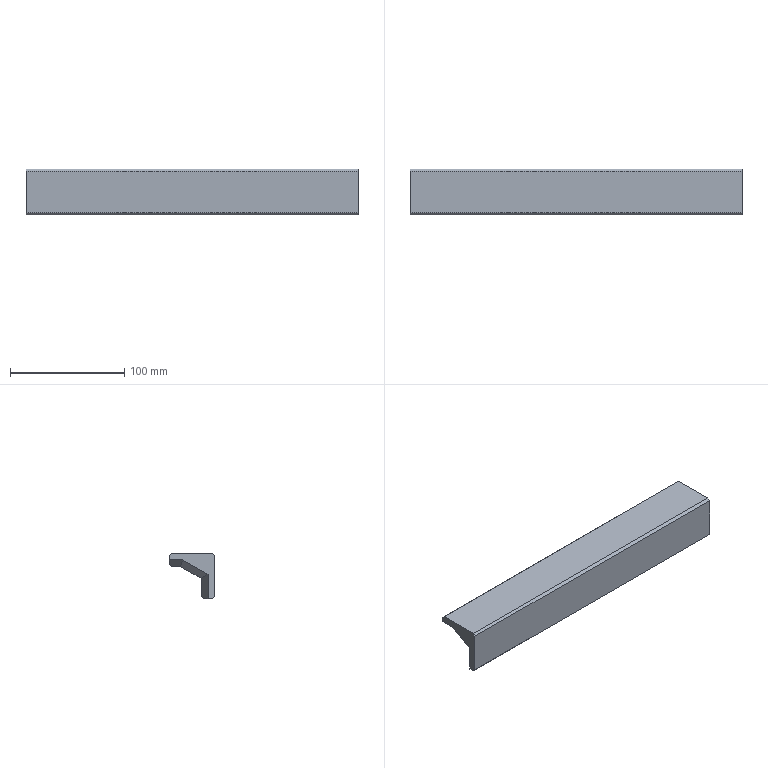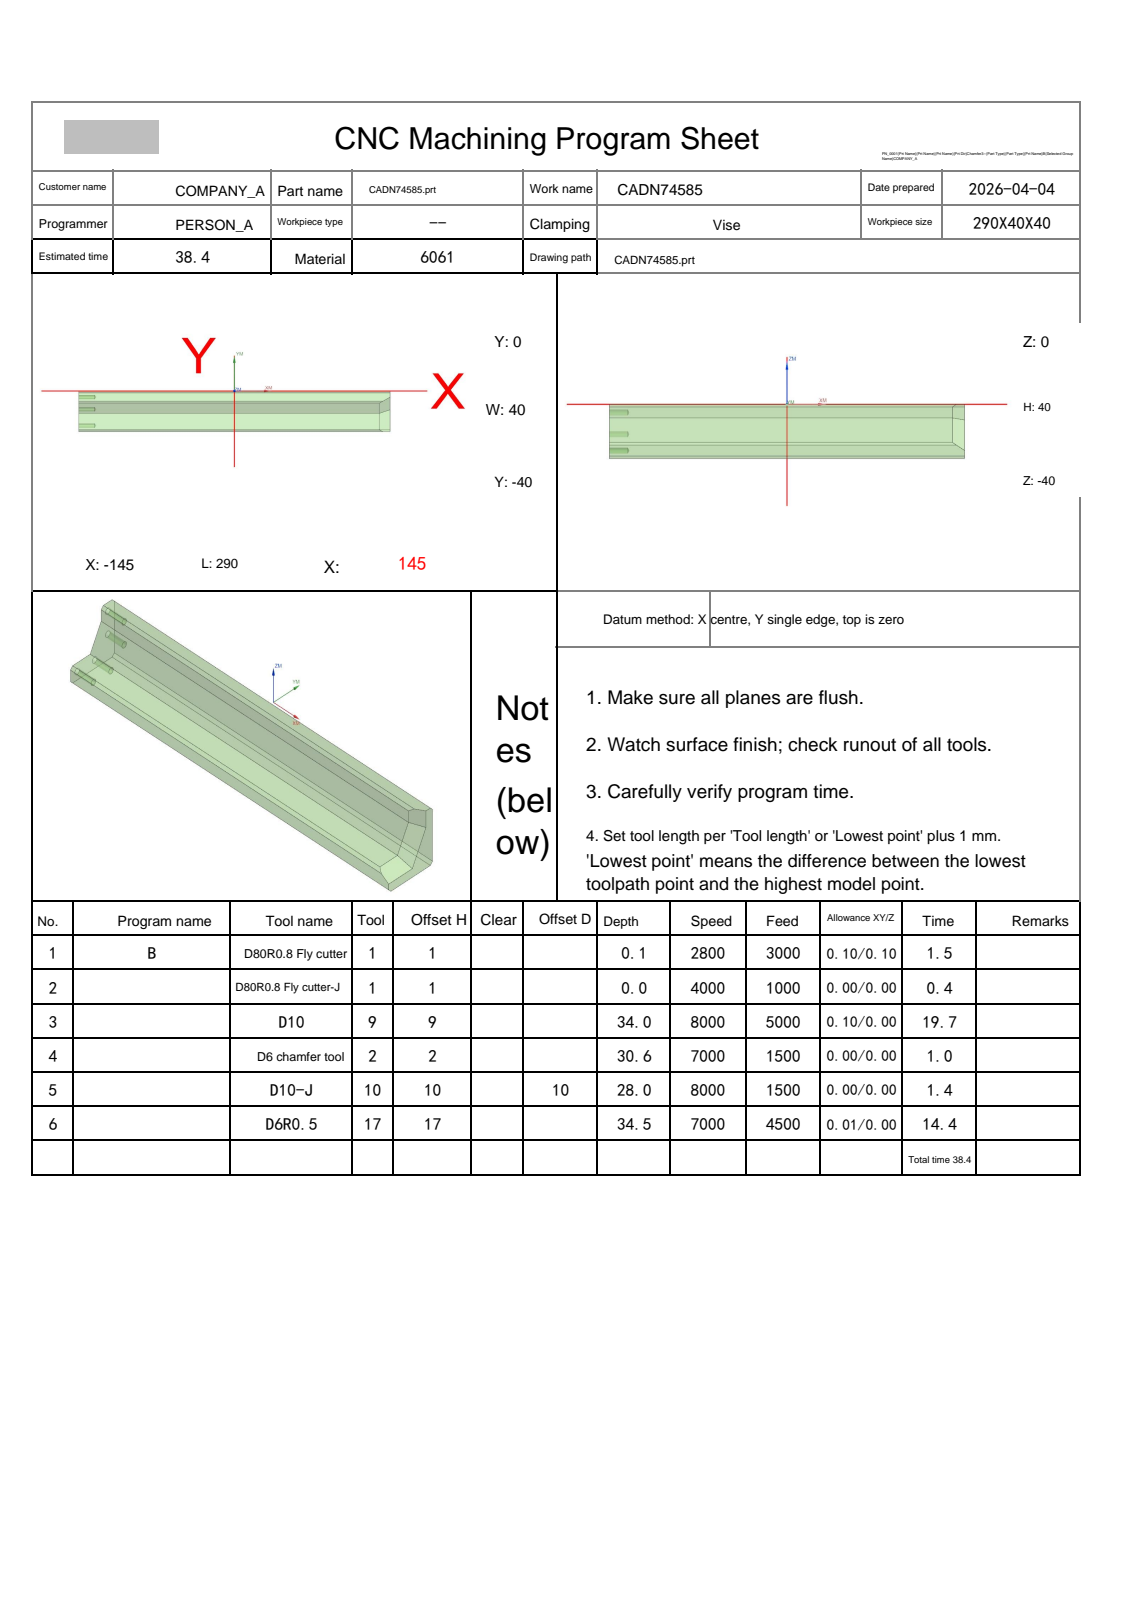NC program | NX | posted by the shop | part box 290 x 40 x 40 mm
Lines 4340 to 6846 of 6846, first 2092 of 2507 lines:
N4 T02 M06
(D6Chamfer D=6. R=0. H=02 ce=0.00 di=0.00)
G00 G90 G54 X-148.9 Y1.516 M03 S6500
G43 H02 Z20.
M08
Z-1.2
G01 Z-2.7 F1000.
G03 X-147.763 Y.7 I1.137 J.384
G01 X147.763
G03 X148.9 Y1.516 I0.0 J1.2
G01 Z-1.2
G00 Z20.
X140.284 Y-13.378
Z-1.2
G01 Z-2.7
G03 X139.204 Y-12.7 I-1.08 J-.522
G01 X-147.763
G03 X-148.9 Y-13.516 I0.0 J-1.2
G01 Z-1.2
G00 Z20.
G00 G90 X142.1 Y-40.6 M03 S7000
Z20.
Z-28.1
G01 Z-30.6 F1000.
X135.
X-145.
X-152.1
Z-28.1
G00 Z20.
G00 G90 X145.99 Y-1.208 M03 S6500
Z20.
Z.13
G01 Z-1.2 F1500.
G03 X145.915 Y-1.548 I1.907 J-.601
G01 X145.905 Y-1.602
X145.928 Y-1.651
X145.966 Y-1.741
X146. Y-2.
Y-6.
X145.967 Y-6.255
X145.87 Y-6.493
X145.716 Y-6.698
X145.514 Y-6.857
X138.848 Y-10.857
X138.6 Y-10.964
X138.534 Y-10.973
X138.51 Y-10.969
X138.495 Y-10.989
X138.435 Y-11.027
X138.393 Y-11.083
Z.314
G00 Z10.
X-145.99 Y-10.792
Z.13
G01 Z-1.2
G03 X-145.915 Y-10.452 I-1.907 J.601
G01 X-145.905 Y-10.398
X-145.928 Y-10.349
X-145.966 Y-10.259
X-146. Y-10.
Y-2.
X-145.966 Y-1.741
X-145.928 Y-1.651
X-145.905 Y-1.602
X-145.915 Y-1.548
G03 X-145.99 Y-1.208 I-1.983 J-.261
G01 Z.13
G00 Z10.
X-145.916 Y-38.379
Z-25.199
G01 Z-29.199
X-145.966 Y-38.259
X-146. Y-38.
Y-24.
X-146.008 Y-23.97
X-146.068 Y-23.884
Z-26.228
G00 Z20.
G91 G28 Z0.0
M05
M09
G91 G28 Z0.0
M01
N5 T10 M06
(D10-J  D=10. R=0. H=10 ce=0.00 di=0.00)
G00 G90 G54 X149.655 Y-10.817 M03 S8000
G43 H10 Z9.5
M08
Z-9.
G01 Z-10. F1000.
G41 D10
X149.533 Y-10.659
G03 X148.344 Y-10.074 I-1.189 J-.915
X147.572 Y-10.287 I0.0 J-1.5
G01 X137.572 Y-16.287
G02 X135. Y-17. I-2.572 J4.287
G01 X-145.
G03 X-146.49 Y-18.327 I0.0 J-1.5
G01 G40 X-146.513 Y-18.526
Z-9.
G00 Z9.5
G00 G90 X142. Y-40.999 M03 S7000
Z14.5
Z-26.5
G01 Z-28. F1500.
G03 X140. Y-39. I-2. J-.001
G01 X-149.1
G02 X-150. Y-38.1 I0.0 J.9
G01 Y-36.133
G02 X-149. Y-35.133 I1. J0.0
G01 X139.1
G03 X140. Y-34.233 I0.0 J.9
G01 Y-32.267
G03 X139. Y-31.267 I-1. J0.0
G01 X-149.1
G02 X-150. Y-30.367 I0.0 J.9
G01 Y-28.4
G02 X-149. Y-27.4 I1. J0.0
G01 X140.
G02 X142. Y-29.399 I0.0 J-2.
G01 Z-26.5
G00 Z14.5
G00 G90 X140.282 Y-27.01 M03 S8000
Z14.5
Z-27.
G01 Z-28. F1000.
G41 D10
X140.083 Y-27.002
X140. Y-27.
X-150.
G03 X-152. Y-28.999 I0.0 J-2.
G01 G40 Y-29.199
Z-27.
G00 Z14.5
G91 G28 Z0.0
M05
M09
G91 G28 Z0.0
M01
N6 T17 M06
(D6R0.5  D=6. R=0.5 H=17 ce=0.01 di=0.00)
G00 G90 G54 X151.954 Y-5.333 M03 S7000
G43 H17 Z14.5
M08
Z-9.6
G01 Z-10.1 F4500.
X147.471 Y-8.027
X146.549 Y-8.581
X136.549 Y-14.581
G02 X135. Y-15.01 I-1.549 J2.581
G01 X-145.
X-146.05
X-146.094 Y-15.008
Z-10.2
X-146.05 Y-15.01
X-145.
X135.
G03 X136.549 Y-14.581 I0.0 J3.01
G01 X146.537 Y-8.588
X146.549 Y-8.582
X147.437 Y-8.05
X147.472 Y-8.027
X147.473 Y-8.028 Z-10.3
X147.437 Y-8.052
X146.538 Y-8.59
X146.482 Y-8.621
X136.549 Y-14.581
G02 X135. Y-15.01 I-1.549 J2.581
G01 X-145.
X-146.05
X-146.095 Y-15.008
Y-15.011 Z-10.348
X-146.096 Y-15.022 Z-10.396
X-146.05 Y-15.024
X135.
G03 X136.553 Y-14.579 I-.028 J3.026
G01 X146.482 Y-8.621
X146.573 Y-8.572
X147.437 Y-8.054
X147.474 Y-8.03
X147.475 Y-8.031 Z-10.484
X146.54 Y-8.592
X146.482 Y-8.621
X137.223 Y-14.176
X136.678 Y-14.551
G02 X135. Y-15.073 I-1.68 J2.443
G01 X-146.05
X-146.098 Y-15.071
X-146.099 Y-15.097 Z-10.527
X-146.1 Y-15.119 Z-10.571
X-146.05 Y-15.121
X135.
G03 X136.678 Y-14.599 I-.003 J2.965
G01 X137.786 Y-13.839
X146.537 Y-8.588
X146.574 Y-8.574
X147.476 Y-8.032
X147.478 Y-8.033 Z-10.658
X147.437 Y-8.06
X146.743 Y-8.476
X146.592 Y-8.565
X146.57 Y-8.568
X138.348 Y-13.502
X136.678 Y-14.648
G02 X135. Y-15.17 I-1.68 J2.443
G01 X-146.05
X-146.1 Y-15.168
Y-15.194 Z-10.702
Y-15.216 Z-10.746
X-146.05 Y-15.219
X135.
G03 X136.678 Y-14.696 I-.003 J2.965
G01 X138.91 Y-13.164
X146.57 Y-8.568
X146.592 Y-8.566
X146.743 Y-8.478
X147.437 Y-8.062
X147.479 Y-8.034
X147.48 Y-8.036 Z-10.833
X147.437 Y-8.064
X146.623 Y-8.55
X146.592 Y-8.566
X146.57 Y-8.568
X139.472 Y-12.827
X136.678 Y-14.745
G02 X135. Y-15.267 I-1.68 J2.443
G01 X-146.05
X-146.1 Y-15.265
Y-15.291 Z-10.877
Y-15.314 Z-10.921
X-146.05 Y-15.316
X135.
G03 X136.678 Y-14.794 I-.003 J2.965
G01 X140.035 Y-12.489
X146.57 Y-8.568
X146.592 Y-8.566
X146.743 Y-8.482
X147.481 Y-8.037
X147.482 Y-8.038 Z-11.008
X147.437 Y-8.067
X146.743 Y-8.484
X146.61 Y-8.558
X146.57 Y-8.568
X140.597 Y-12.152
X136.678 Y-14.842
G02 X135. Y-15.364 I-1.68 J2.443
G01 X-146.05
X-146.1 Y-15.362
Y-15.389 Z-11.052
Y-15.411 Z-11.095
X-146.05 Y-15.413
X135.
G03 X136.678 Y-14.891 I-.003 J2.965
G01 X141.159 Y-11.815
X146.549 Y-8.581
X146.587 Y-8.558
X146.61
X146.743 Y-8.486
X147.437 Y-8.069
X147.483 Y-8.039
X147.484 Y-8.04 Z-11.183
X147.437 Y-8.071
X146.743 Y-8.487
X146.61 Y-8.558
X146.587
X146.549 Y-8.581
X141.721 Y-11.477
X136.678 Y-14.939
G02 X135. Y-15.461 I-1.68 J2.443
G01 X-146.05
X-146.1 Y-15.459
Y-15.486 Z-11.227
Y-15.508 Z-11.27
X-146.05 Y-15.51
X135.
G03 X136.678 Y-14.988 I-.003 J2.965
G01 X142.284 Y-11.14
X146.549 Y-8.581
X146.587 Y-8.558
X146.61
X146.743 Y-8.488
X147.437 Y-8.073
X147.485 Y-8.041
X147.486 Y-8.043 Z-11.358
X147.437 Y-8.075
X146.743 Y-8.489
X146.61 Y-8.558
X146.587
X146.549 Y-8.581
X142.846 Y-10.803
X136.678 Y-15.036
G02 X135. Y-15.558 I-1.68 J2.443
G01 X-146.05
X-146.1 Y-15.556
Y-15.583 Z-11.401
Y-15.605 Z-11.445
X-146.05 Y-15.607
X135.
G03 X136.678 Y-15.085 I-.003 J2.965
G01 X143.408 Y-10.465
X146.549 Y-8.581
X146.587 Y-8.558
X146.61
X146.743 Y-8.49
X147.437 Y-8.077
X147.488 Y-8.044
X147.489 Y-8.045 Z-11.533
X146.743 Y-8.49
X146.624 Y-8.551
X146.603 Y-8.547
X146.549 Y-8.581
X143.97 Y-10.128
X136.678 Y-15.134
G02 X135. Y-15.656 I-1.68 J2.443
G01 X-146.05
X-146.1 Y-15.653
Y-15.68 Z-11.576
Y-15.702 Z-11.62
X-146.05 Y-15.704
X135.
G03 X136.678 Y-15.182 I-.003 J2.965
G01 X144.533 Y-9.791
X146.549 Y-8.581
X146.603 Y-8.547
X146.624 Y-8.551
X146.743 Y-8.49
X147.437 Y-8.081
X147.49 Y-8.046
X147.491 Y-8.047 Z-11.707
X147.437 Y-8.083
X146.743 Y-8.491
X146.624 Y-8.551
X146.603 Y-8.547
X146.549 Y-8.581
X145.095 Y-9.453
X136.678 Y-15.231
G02 X135. Y-15.753 I-1.68 J2.443
G01 X-146.05
X-146.1 Y-15.751
Y-15.777 Z-11.751
Y-15.799 Z-11.795
X-146.05 Y-15.801
X135.
G03 X136.678 Y-15.279 I-.003 J2.965
G01 X145.657 Y-9.116
X146.549 Y-8.581
X146.603 Y-8.547
X146.624 Y-8.551
G03 X147.492 Y-8.048 I-3.924 J7.775
G01 X147.493 Y-8.05 Z-11.882
G02 X146.624 Y-8.551 I-4.828 J7.36
G01 X146.603 Y-8.547
X146.549 Y-8.581
X146.219 Y-8.779
X136.678 Y-15.328
G02 X135. Y-15.85 I-1.68 J2.443
G01 X-146.05
X-146.1 Y-15.848
Y-15.874 Z-11.926
Y-15.896 Z-11.97
X-146.05 Y-15.898
X135.
G03 X136.678 Y-15.376 I-.003 J2.965
G01 X146.602 Y-8.564
G03 X147.495 Y-8.051 I-4.612 J9.049
G01 X147.496 Y-8.052 Z-12.057
G02 X146.633 Y-8.592 I-5.008 J7.049
G01 X136.678 Y-15.425
G02 X135. Y-15.947 I-1.68 J2.443
G01 X-146.05
X-146.1 Y-15.945
Y-15.971 Z-12.101
Y-15.993 Z-12.144
X-146.05 Y-15.996
X135.
G03 X136.678 Y-15.474 I-.003 J2.965
G01 X146.655 Y-8.625
G03 X147.512 Y-8.083 I-3.927 J7.161
G01 X147.524 Y-8.1 Z-12.188
X147.534 Y-8.114 Z-12.232
G02 X146.678 Y-8.658 I-4.667 J6.402
G01 X136.678 Y-15.522
G02 X135. Y-16.044 I-1.68 J2.443
G01 X-146.05
X-146.1 Y-16.042
Y-16.068 Z-12.276
Y-16.091 Z-12.319
X-146.05 Y-16.093
X135.
G03 X136.678 Y-15.571 I-.003 J2.965
G01 X146.636 Y-8.735
G03 X147.556 Y-8.146 I-6.747 J11.544
G01 X147.568 Y-8.162 Z-12.363
X147.579 Y-8.178 Z-12.407
X147.549 Y-8.199
X147.09 Y-8.509
X147.032 Y-8.544
X146.707 Y-8.736
X146.646 Y-8.777
X136.678 Y-15.619
G02 X135. Y-16.141 I-1.68 J2.443
G01 X-146.05
X-146.1 Y-16.139
Y-16.166 Z-12.45
Y-16.188 Z-12.494
X-146.05 Y-16.19
X135.
G03 X136.678 Y-15.668 I-.003 J2.965
G01 X146.655 Y-8.819
X146.729 Y-8.769
X147.09 Y-8.555
X147.595 Y-8.213
X147.596 Y-8.257 Z-12.582
X147.09 Y-8.601
G03 X146.65 Y-8.871 I1.947 J-3.669
G01 X136.678 Y-15.716
G02 X135. Y-16.238 I-1.68 J2.443
G01 X-146.05
X-146.1 Y-16.236
Y-16.263 Z-12.625
Y-16.285 Z-12.669
X-146.05 Y-16.287
X135.
G03 X136.678 Y-15.765 I-.003 J2.965
G01 X146.7 Y-8.886
G02 X147.09 Y-8.648 I2.403 J-3.501
G01 X147.598 Y-8.302
X147.599 Y-8.347 Z-12.756
X147.09 Y-8.694
G03 X146.679 Y-8.949 I2.522 J-4.53
G01 X136.678 Y-15.813
G02 X135. Y-16.336 I-1.68 J2.443
G01 X-146.05
X-146.1 Y-16.333
Y-16.36 Z-12.8
Y-16.382 Z-12.844
X-146.05 Y-16.384
X135.
G03 X136.678 Y-15.862 I-.003 J2.965
G01 X146.652 Y-9.016
G02 X147.09 Y-8.74 I3.675 J-5.354
G01 X147.601 Y-8.392
X147.603 Y-8.437 Z-12.931
X147.09 Y-8.786
G03 X146.656 Y-9.062 I3.569 J-6.109
G01 X136.678 Y-15.911
G02 X135. Y-16.433 I-1.68 J2.443
G01 X-146.05
X-146.1 Y-16.43
Y-16.457 Z-12.975
Y-16.48 Z-13.019
X-146.05 Y-16.481
X135.
G03 X136.678 Y-15.959 I-.003 J2.965
G01 X146.664 Y-9.105
G02 X147.09 Y-8.832 I4.332 J-6.312
G01 X147.519 Y-8.544
X147.605 Y-8.483
X147.608 Y-8.529 Z-13.106
X147.437 Y-8.646
X146.546 Y-9.234
X136.678 Y-16.008
G02 X135. Y-16.53 I-1.68 J2.443
G01 X-146.05
X-146.1 Y-16.528
Y-16.554 Z-13.15
Y-16.576 Z-13.193
X-146.05 Y-16.578
X135.
G03 X136.678 Y-16.056 I-.003 J2.965
G01 X146.667 Y-9.2
X147.437 Y-8.692
X147.609 Y-8.574
X147.61 Y-8.618 Z-13.281
X147.437 Y-8.739
X146.669 Y-9.247
X136.678 Y-16.105
G02 X135. Y-16.627 I-1.68 J2.443
G01 X-146.05
X-146.1 Y-16.625
Y-16.651 Z-13.325
Y-16.673 Z-13.368
X-146.05 Y-16.675
X135.
G03 X136.678 Y-16.153 I-.003 J2.965
G01 X146.678 Y-9.29
X147.437 Y-8.785
X147.611 Y-8.663
X147.613 Y-8.708 Z-13.456
X146.678 Y-9.338
X136.678 Y-16.202
G02 X135. Y-16.724 I-1.68 J2.443
G01 X-146.05
X-146.1 Y-16.722
Y-16.748 Z-13.499
Y-16.77 Z-13.543
X-146.05 Y-16.773
X135.
G03 X136.678 Y-16.251 I-.003 J2.965
G01 X146.678 Y-9.387
X147.437 Y-8.877
X147.615 Y-8.753
X147.617 Y-8.799 Z-13.631
X147.488 Y-8.889
X146.678 Y-9.435
X136.678 Y-16.299
G02 X135. Y-16.821 I-1.68 J2.443
G01 X-146.05
X-146.1 Y-16.819
Y-16.845 Z-13.674
Y-16.868 Z-13.718
X-146.05 Y-16.87
X135.
G03 X136.678 Y-16.348 I-.003 J2.965
G01 X146.678 Y-9.484
X147.557 Y-8.889
X147.62 Y-8.845
X147.622 Y-8.892 Z-13.805
X146.678 Y-9.532
X136.678 Y-16.396
G02 X135. Y-16.918 I-1.68 J2.443
G01 X-146.05
X-146.1 Y-16.916
Y-16.943 Z-13.849
Y-16.965 Z-13.893
X-146.05 Y-16.967
X135.
G03 X136.678 Y-16.445 I-.003 J2.965
G01 X146.678 Y-9.581
X147.437 Y-9.067
X147.621 Y-8.938
X147.62 Y-8.985 Z-13.98
X147.437 Y-9.115
X146.678 Y-9.63
X136.678 Y-16.493
G02 X135. Y-17.015 I-1.68 J2.443
G01 X-146.05
X-146.1 Y-17.013
Y-17.04 Z-14.024
Y-17.062 Z-14.068
X-146.05 Y-17.064
X135.
G03 X136.678 Y-16.542 I-.003 J2.965
G01 X146.678 Y-9.678
X147.437 Y-9.162
X147.62 Y-9.033
Y-9.08 Z-14.155
X147.437 Y-9.209
X146.678 Y-9.727
X136.678 Y-16.59
G02 X135. Y-17.113 I-1.68 J2.443
G01 X-146.05
X-146.1 Y-17.11
Y-17.137 Z-14.199
Y-17.159 Z-14.242
X-146.05 Y-17.161
X135.
G03 X136.678 Y-16.639 I-.003 J2.965
G01 X146.678 Y-9.775
X147.471 Y-9.234
X147.62 Y-9.129
X147.621 Y-9.178 Z-14.33
X147.543 Y-9.234
X146.678 Y-9.824
X136.678 Y-16.688
G02 X135. Y-17.21 I-1.68 J2.443
G01 X-146.05
X-146.1 Y-17.208
Y-17.234 Z-14.374
Y-17.256 Z-14.417
X-146.05 Y-17.258
X135.
G03 X136.678 Y-16.736 I-.003 J2.965
G01 X146.678 Y-9.872
X147.622 Y-9.228
X147.621 Y-9.275 Z-14.505
X147.437 Y-9.402
X146.678 Y-9.921
X136.678 Y-16.785
G02 X135. Y-17.307 I-1.68 J2.443
G01 X-146.05
X-146.1 Y-17.305
Y-17.331 Z-14.548
Y-17.353 Z-14.592
X-146.05 Y-17.355
X135.
G03 X136.678 Y-16.833 I-.003 J2.965
G01 X146.678 Y-9.97
X147.437 Y-9.45
X147.62 Y-9.322
Y-9.37 Z-14.68
X147.437 Y-9.499
X146.678 Y-10.018
X136.678 Y-16.882
G02 X135. Y-17.404 I-1.68 J2.443
G01 X-146.05
X-146.1 Y-17.402
Y-17.428 Z-14.723
Y-17.45 Z-14.767
X-146.05 Y-17.453
X135.
G03 X136.678 Y-16.93 I-.003 J2.965
G01 X146.678 Y-10.067
X147.437 Y-9.547
X147.62 Y-9.418
Y-9.467 Z-14.854
X147.461 Y-9.579
X146.678 Y-10.115
X136.678 Y-16.979
G02 X135. Y-17.501 I-1.68 J2.443
G01 X-146.05
X-146.1 Y-17.499
Y-17.525 Z-14.898
Y-17.547 Z-14.942
X-146.05 Y-17.55
X135.
G03 X136.678 Y-17.028 I-.003 J2.965
G01 X146.678 Y-10.164
X147.532 Y-9.579
X147.62 Y-9.516
X147.621 Y-9.566 Z-15.029
X146.678 Y-10.212
X136.678 Y-17.076
G02 X135. Y-17.598 I-1.68 J2.443
G01 X-146.05
X-146.1 Y-17.596
Y-17.622 Z-15.073
Y-17.645 Z-15.117
X-146.05 Y-17.647
X135.
G03 X136.678 Y-17.125 I-.003 J2.965
G01 X146.678 Y-10.261
X147.437 Y-9.74
X147.62 Y-9.614
Y-9.661 Z-15.204
X147.437 Y-9.789
X146.678 Y-10.309
X136.678 Y-17.173
G02 X135. Y-17.695 I-1.68 J2.443
G01 X-146.05
X-146.1 Y-17.693
Y-17.72 Z-15.248
Y-17.742 Z-15.291
X-146.05 Y-17.744
X135.
G03 X136.678 Y-17.222 I-.003 J2.965
G01 X146.678 Y-10.358
X147.437 Y-9.837
X147.619 Y-9.709
Y-9.757 Z-15.379
X147.437 Y-9.886
X146.678 Y-10.407
X136.678 Y-17.27
G02 X135. Y-17.792 I-1.68 J2.443
G01 X-146.05
X-146.1 Y-17.79
Y-17.817 Z-15.423
Y-17.839 Z-15.466
X-146.05 Y-17.841
X135.
G03 X136.678 Y-17.319 I-.003 J2.965
G01 X146.678 Y-10.455
X147.452 Y-9.924
X147.619 Y-9.806
Y-9.855 Z-15.554
X147.522 Y-9.924
X146.678 Y-10.504
X136.678 Y-17.368
G02 X135. Y-17.89 I-1.68 J2.443
G01 X-146.05
X-146.1 Y-17.887
Y-17.914 Z-15.597
Y-17.936 Z-15.641
X-146.05 Y-17.938
X135.
G03 X136.678 Y-17.416 I-.003 J2.965
G01 X146.678 Y-10.552
X147.593 Y-9.924
X147.62 Y-9.904
Y-9.953 Z-15.729
X147.437 Y-10.08
X146.678 Y-10.601
X136.678 Y-17.465
G02 X135. Y-17.987 I-1.68 J2.443
G01 X-146.05
X-146.1 Y-17.985
Y-18.011 Z-15.772
Y-18.033 Z-15.816
X-146.05 Y-18.035
X135.
G03 X136.678 Y-17.513 I-.003 J2.965
G01 X146.678 Y-10.649
X147.437 Y-10.128
X147.619 Y-10.
Y-10.048 Z-15.903
X147.437 Y-10.177
X146.678 Y-10.698
X136.678 Y-17.562
G02 X135. Y-18.084 I-1.68 J2.443
G01 X-146.05
X-146.1 Y-18.082
Y-18.108 Z-15.947
Y-18.13 Z-15.991
X-146.05 Y-18.132
X135.
G03 X136.678 Y-17.61 I-.003 J2.965
G01 X146.678 Y-10.747
X147.437 Y-10.225
X147.619 Y-10.097
Y-10.145 Z-16.078
X147.444 Y-10.269
X146.678 Y-10.795
X136.678 Y-17.659
G02 X135. Y-18.181 I-1.68 J2.443
G01 X-146.05
X-146.1 Y-18.179
Y-18.205 Z-16.122
Y-18.227 Z-16.166
X-146.05 Y-18.23
X135.
G03 X136.678 Y-17.707 I-.003 J2.965
G01 X146.678 Y-10.844
X147.515 Y-10.269
X147.619 Y-10.194
X147.62 Y-10.244 Z-16.253
X147.586 Y-10.269
X146.678 Y-10.892
X136.678 Y-17.756
G02 X135. Y-18.278 I-1.68 J2.443
G01 X-146.05
X-146.1 Y-18.276
Y-18.302 Z-16.297
Y-18.325 Z-16.34
X-146.05 Y-18.327
X135.
G03 X136.678 Y-17.805 I-.003 J2.965
G01 X146.678 Y-10.941
X147.437 Y-10.42
X147.62 Y-10.293
X147.619 Y-10.34 Z-16.428
X147.437 Y-10.468
X146.678 Y-10.989
X136.678 Y-17.853
G02 X135. Y-18.375 I-1.68 J2.443
G01 X-146.05
X-146.1 Y-18.373
Y-18.4 Z-16.472
Y-18.422 Z-16.515
X-146.05 Y-18.424
X135.
G03 X136.678 Y-17.902 I-.003 J2.965
G01 X146.678 Y-11.038
X147.437 Y-10.517
X147.619 Y-10.388
Y-10.436 Z-16.603
X147.437 Y-10.565
X146.678 Y-11.087
X136.678 Y-17.95
G02 X135. Y-18.472 I-1.68 J2.443
G01 X-146.05
X-146.1 Y-18.47
Y-18.497 Z-16.646
Y-18.519 Z-16.69
X-146.05 Y-18.521
X135.
G03 X136.678 Y-17.999 I-.003 J2.965
G01 X146.678 Y-11.135
X147.437 Y-10.614
X147.619 Y-10.485
Y-10.534 Z-16.778
X147.507 Y-10.614
X146.678 Y-11.184
X136.678 Y-18.047
G02 X135. Y-18.569 I-1.68 J2.443
G01 X-146.05
X-146.1 Y-18.567
Y-18.594 Z-16.821
Y-18.616 Z-16.865
X-146.05 Y-18.618
X135.
G03 X136.678 Y-18.096 I-.003 J2.965
G01 X146.678 Y-11.232
X147.578 Y-10.614
X147.62 Y-10.584
Y-10.633 Z-16.952
X147.437 Y-10.76
X146.678 Y-11.281
X136.678 Y-18.145
G02 X135. Y-18.667 I-1.68 J2.443
G01 X-146.05
X-146.1 Y-18.664
Y-18.691 Z-16.996
Y-18.713 Z-17.04
X-146.05 Y-18.715
X135.
G03 X136.678 Y-18.193 I-.003 J2.965
G01 X146.678 Y-11.329
X147.437 Y-10.808
X147.619 Y-10.68
Y-10.728 Z-17.127
X147.437 Y-10.857
X146.678 Y-11.378
X136.678 Y-18.242
G02 X135. Y-18.764 I-1.68 J2.443
G01 X-146.05
X-146.1 Y-18.762
Y-18.788 Z-17.171
Y-18.81 Z-17.215
X-146.05 Y-18.812
X135.
G03 X136.678 Y-18.29 I-.003 J2.965
G01 X146.678 Y-11.426
X147.437 Y-10.905
X147.619 Y-10.776
Y-10.825 Z-17.302
X147.437 Y-10.954
X146.678 Y-11.475
X136.678 Y-18.339
G02 X135. Y-18.861 I-1.68 J2.443
G01 X-146.05
X-146.1 Y-18.859
Y-18.885 Z-17.346
Y-18.907 Z-17.389
X-146.05 Y-18.909
X135.
G03 X136.678 Y-18.387 I-.003 J2.965
G01 X146.678 Y-11.524
X147.5 Y-10.959
X147.619 Y-10.874
X147.62 Y-10.924 Z-17.477
X147.571 Y-10.959
X146.678 Y-11.572
X136.678 Y-18.436
G02 X135. Y-18.958 I-1.68 J2.443
G01 X-146.05
X-146.1 Y-18.956
Y-18.982 Z-17.521
Y-19.004 Z-17.564
X-146.05 Y-19.007
X135.
G03 X136.678 Y-18.484 I-.003 J2.965
G01 X146.678 Y-11.621
X147.62 Y-10.973
X147.619 Y-11.02 Z-17.652
X147.437 Y-11.148
X146.678 Y-11.669
X136.678 Y-18.533
G02 X135. Y-19.055 I-1.68 J2.443
G01 X-146.05
X-146.1 Y-19.053
Y-19.079 Z-17.695
Y-19.102 Z-17.739
X-146.05 Y-19.104
X135.
G03 X136.678 Y-18.582 I-.003 J2.965
G01 X146.678 Y-11.718
X147.437 Y-11.197
X147.619 Y-11.068
Y-11.116 Z-17.826
X147.437 Y-11.245
X146.678 Y-11.766
X136.678 Y-18.63
G02 X135. Y-19.152 I-1.68 J2.443
G01 X-146.05
X-146.1 Y-19.15
Y-19.177 Z-17.87
Y-19.199 Z-17.914
X-146.05 Y-19.201
X135.
G03 X136.678 Y-18.679 I-.003 J2.965
G01 X146.678 Y-11.815
X147.437 Y-11.294
X147.619 Y-11.165
Y-11.214 Z-18.001
X147.493 Y-11.304
X146.678 Y-11.864
X136.678 Y-18.727
G02 X135. Y-19.249 I-1.68 J2.443
G01 X-146.05
X-146.1 Y-19.247
Y-19.274 Z-18.045
Y-19.296 Z-18.089
X-146.05 Y-19.298
X135.
G03 X136.678 Y-18.776 I-.003 J2.965
G01 X146.678 Y-11.912
X147.563 Y-11.304
X147.62 Y-11.263
X147.621 Y-11.313 Z-18.176
X146.678 Y-11.961
X136.678 Y-18.824
G02 X135. Y-19.347 I-1.68 J2.443
G01 X-146.05
X-146.1 Y-19.344
Y-19.371 Z-18.22
Y-19.393 Z-18.264
X-146.05 Y-19.395
X135.
G03 X136.678 Y-18.873 I-.003 J2.965
G01 X146.678 Y-12.009
X147.437 Y-11.488
X147.62 Y-11.36
X147.619 Y-11.408 Z-18.351
X147.437 Y-11.537
X146.678 Y-12.058
X136.678 Y-18.922
G02 X135. Y-19.444 I-1.68 J2.443
G01 X-146.05
X-146.1 Y-19.441
Y-19.468 Z-18.395
Y-19.49 Z-18.438
X-146.05 Y-19.492
X135.
G03 X136.678 Y-18.97 I-.003 J2.965
G01 X146.678 Y-12.106
X147.437 Y-11.585
X147.619 Y-11.456
Y-11.505 Z-18.526
X147.437 Y-11.634
X146.678 Y-12.155
X136.678 Y-19.019
G02 X135. Y-19.541 I-1.68 J2.443
G01 X-146.05
X-146.1 Y-19.539
Y-19.565 Z-18.57
Y-19.588 Z-18.613
X-146.05 Y-19.589
X135.
G03 X136.678 Y-19.067 I-.003 J2.965
G01 X146.678 Y-12.203
X147.485 Y-11.649
X147.619 Y-11.554
X147.62 Y-11.603 Z-18.701
X147.556 Y-11.649
X146.678 Y-12.252
X136.678 Y-19.116
G02 X135. Y-19.638 I-1.68 J2.443
G01 X-146.05
X-146.1 Y-19.636
Y-19.662 Z-18.744
Y-19.684 Z-18.788
X-146.05 Y-19.686
X135.
G03 X136.678 Y-19.164 I-.003 J2.965
G01 X146.678 Y-12.301
X147.621 Y-11.653
X147.62 Y-11.7 Z-18.875
X147.437 Y-11.828
X146.678 Y-12.349
X136.678 Y-19.213
G02 X135. Y-19.735 I-1.68 J2.443
G01 X-146.05
X-146.1 Y-19.733
Y-19.759 Z-18.919
Y-19.781 Z-18.963
X-146.05 Y-19.784
X135.
G03 X136.678 Y-19.262 I-.003 J2.965
G01 X146.678 Y-12.398
X147.437 Y-11.877
X147.619 Y-11.748
Y-11.796 Z-19.05
X147.437 Y-11.925
X146.678 Y-12.446
X136.678 Y-19.31
G02 X135. Y-19.832 I-1.68 J2.443
G01 X-146.05
X-146.1 Y-19.83
Y-19.856 Z-19.094
Y-19.879 Z-19.138
X-146.05 Y-19.881
X135.
G03 X136.678 Y-19.359 I-.003 J2.965
G01 X146.678 Y-12.495
X147.437 Y-11.974
X147.619 Y-11.845
Y-11.894 Z-19.225
X147.478 Y-11.994
X146.678 Y-12.543
X136.678 Y-19.407
G02 X135. Y-19.929 I-1.68 J2.443
G01 X-146.05
X-146.1 Y-19.927
Y-19.954 Z-19.269
Y-19.976 Z-19.313
X-146.05 Y-19.978
X135.
G03 X136.678 Y-19.456 I-.003 J2.965
G01 X146.678 Y-12.592
X147.549 Y-11.994
X147.62 Y-11.943
X147.621 Y-11.993 Z-19.4
X146.678 Y-12.641
X136.678 Y-19.504
G02 X135. Y-20.026 I-1.68 J2.443
G01 X-146.05
X-146.1 Y-20.024
Y-20.051 Z-19.444
Y-20.073 Z-19.487
X-146.05 Y-20.075
X135.
G03 X136.678 Y-19.553 I-.003 J2.965
G01 X146.678 Y-12.689
X147.437 Y-12.168
X147.62 Y-12.04
X147.619 Y-12.088 Z-19.575
X147.437 Y-12.216
X146.678 Y-12.738
X136.678 Y-19.601
G02 X135. Y-20.124 I-1.68 J2.443
G01 X-146.05
X-146.1 Y-20.121
Y-20.148 Z-19.619
Y-20.17 Z-19.662
X-146.05 Y-20.172
X135.
G03 X136.678 Y-19.65 I-.003 J2.965
G01 X146.678 Y-12.786
X147.437 Y-12.265
X147.619 Y-12.136
Y-12.185 Z-19.75
X147.437 Y-12.314
X146.678 Y-12.835
X136.678 Y-19.699
G02 X135. Y-20.221 I-1.68 J2.443
G01 X-146.05
X-146.1 Y-20.219
Y-20.245 Z-19.793
Y-20.267 Z-19.837
X-146.05 Y-20.269
X135.
G03 X136.678 Y-19.747 I-.003 J2.965
G01 X146.678 Y-12.883
X147.47 Y-12.339
X147.619 Y-12.233
X147.62 Y-12.283 Z-19.924
X147.541 Y-12.339
X146.678 Y-12.932
X136.678 Y-19.796
G02 X135. Y-20.318 I-1.68 J2.443
G01 X-146.05
X-146.1 Y-20.316
Y-20.342 Z-19.968
Y-20.364 Z-20.012
X-146.05 Y-20.366
X135.
G03 X136.678 Y-19.844 I-.003 J2.965
G01 X146.678 Y-12.981
X147.621 Y-12.333
X147.62 Y-12.38 Z-20.099
X147.437 Y-12.508
X146.397 Y-13.222
X136.678 Y-19.893
G02 X135. Y-20.415 I-1.68 J2.443
G01 X-146.05
X-146.1 Y-20.413
Y-20.439 Z-20.143
Y-20.461 Z-20.187
X-146.05 Y-20.463
X135.
G03 X136.678 Y-19.941 I-.003 J2.965
G01 X146.678 Y-13.078
X147.437 Y-12.556
X147.619 Y-12.428
Y-12.476 Z-20.274
X147.437 Y-12.605
X146.678 Y-13.126
X136.678 Y-19.99
G02 X135. Y-20.512 I-1.68 J2.443
G01 X-146.05
X-146.1 Y-20.51
Y-20.536 Z-20.318
Y-20.558 Z-20.362
X-146.05 Y-20.561
X135.
G03 X136.678 Y-20.039 I-.003 J2.965
G01 X146.678 Y-13.175
X147.437 Y-12.654
X147.619 Y-12.525
Y-12.573 Z-20.449
X147.463 Y-12.684
X146.678 Y-13.223
X136.678 Y-20.087
G02 X135. Y-20.609 I-1.68 J2.443
G01 X-146.05
X-146.1 Y-20.607
Y-20.633 Z-20.493
Y-20.656 Z-20.536
X-146.05 Y-20.658
X135.
G03 X136.678 Y-20.136 I-.003 J2.965
G01 X146.678 Y-13.272
X147.534 Y-12.684
X147.62 Y-12.623
X147.621 Y-12.673 Z-20.624
X146.678 Y-13.32
X136.678 Y-20.184
G02 X135. Y-20.706 I-1.68 J2.443
G01 X-146.05
X-146.1 Y-20.704
Y-20.731 Z-20.668
Y-20.753 Z-20.711
X-146.05 Y-20.755
X135.
G03 X136.678 Y-20.233 I-.003 J2.965
G01 X146.678 Y-13.369
X147.437 Y-12.848
X147.62 Y-12.72
X147.619 Y-12.768 Z-20.799
X147.437 Y-12.896
X146.678 Y-13.418
X136.678 Y-20.281
G02 X135. Y-20.803 I-1.68 J2.443
G01 X-146.05
X-146.1 Y-20.801
Y-20.828 Z-20.842
Y-20.85 Z-20.886
X-146.05 Y-20.852
X135.
G03 X136.678 Y-20.33 I-.003 J2.965
G01 X146.678 Y-13.466
X147.437 Y-12.945
X147.619 Y-12.816
Y-12.865 Z-20.973
X147.437 Y-12.993
X146.678 Y-13.515
X136.678 Y-20.379
G02 X135. Y-20.901 I-1.68 J2.443
G01 X-146.05
X-146.1 Y-20.898
Y-20.925 Z-21.017
Y-20.947 Z-21.061
X-146.05 Y-20.949
X135.
G03 X136.678 Y-20.427 I-.003 J2.965
G01 X146.678 Y-13.563
X147.456 Y-13.029
X147.619 Y-12.913
Y-12.963 Z-21.148
X147.526 Y-13.029
X146.678 Y-13.612
X136.678 Y-20.476
G02 X135. Y-20.998 I-1.68 J2.443
G01 X-146.05
X-146.1 Y-20.996
Y-21.022 Z-21.192
Y-21.044 Z-21.236
X-146.05 Y-21.046
X135.
G03 X136.678 Y-20.524 I-.003 J2.965
G01 X146.678 Y-13.66
X147.62 Y-13.012
Y-13.061 Z-21.323
X147.437 Y-13.188
X146.678 Y-13.709
X136.678 Y-20.573
G02 X135. Y-21.095 I-1.68 J2.443
G01 X-146.05
X-146.1 Y-21.093
Y-21.119 Z-21.367
Y-21.141 Z-21.411
X-146.05 Y-21.143
X135.
G03 X136.678 Y-20.621 I-.003 J2.965
G01 X146.678 Y-13.758
X147.437 Y-13.236
X147.619 Y-13.108
Y-13.156 Z-21.498
X147.437 Y-13.285
X146.678 Y-13.806
X136.678 Y-20.67
G02 X135. Y-21.192 I-1.68 J2.443
G01 X-146.05
X-146.1 Y-21.19
Y-21.216 Z-21.542
Y-21.238 Z-21.585
X-146.05 Y-21.241
X135.
G03 X136.678 Y-20.718 I-.003 J2.965
G01 X146.678 Y-13.855
X147.437 Y-13.333
X147.619 Y-13.205
Y-13.253 Z-21.673
X147.448 Y-13.375
X146.678 Y-13.903
X136.678 Y-20.767
G02 X135. Y-21.289 I-1.68 J2.443
G01 X-146.05
X-146.1 Y-21.287
Y-21.313 Z-21.716
Y-21.335 Z-21.76
X-146.05 Y-21.338
X135.
G03 X136.678 Y-20.816 I-.003 J2.965
G01 X146.678 Y-13.952
X147.519 Y-13.375
X147.619 Y-13.302
X147.62 Y-13.352 Z-21.848
X147.59 Y-13.375
X146.678 Y-14.
X136.678 Y-20.864
G02 X135. Y-21.386 I-1.68 J2.443
G01 X-146.05
X-146.1 Y-21.384
Y-21.41 Z-21.891
Y-21.433 Z-21.935
X-146.05 Y-21.435
X135.
G03 X136.678 Y-20.913 I-.003 J2.965
G01 X146.678 Y-14.049
X147.437 Y-13.528
X147.62 Y-13.401
X147.619 Y-13.448 Z-22.022
X147.437 Y-13.576
X146.678 Y-14.097
X136.678 Y-20.961
G02 X135. Y-21.483 I-1.68 J2.443
G01 X-146.05
X-146.1 Y-21.481
Y-21.508 Z-22.066
Y-21.53 Z-22.11
X-146.05 Y-21.532
X135.
G03 X136.678 Y-21.01 I-.003 J2.965
G01 X146.678 Y-14.146
X147.437 Y-13.625
X147.619 Y-13.496
Y-13.544 Z-22.197
X147.437 Y-13.673
X146.678 Y-14.195
X136.678 Y-21.058
G02 X135. Y-21.58 I-1.68 J2.443
G01 X-146.05
X-146.1 Y-21.578
Y-21.605 Z-22.241
Y-21.627 Z-22.285
X-146.05 Y-21.629
X135.
G03 X136.678 Y-21.107 I-.003 J2.965
G01 X146.678 Y-14.243
X147.441 Y-13.72
X147.619 Y-13.593
Y-13.642 Z-22.372
X147.512 Y-13.72
X146.678 Y-14.292
X136.678 Y-21.156
G02 X135. Y-21.678 I-1.68 J2.443
G01 X-146.05
X-146.1 Y-21.675
Y-21.702 Z-22.416
Y-21.724 Z-22.46
X-146.05 Y-21.726
X135.
G03 X136.678 Y-21.204 I-.003 J2.965
G01 X146.678 Y-14.34
X147.582 Y-13.72
X147.62 Y-13.692
Y-13.741 Z-22.547
X147.437 Y-13.868
X146.678 Y-14.389
X136.678 Y-21.253
G02 X135. Y-21.775 I-1.68 J2.443
G01 X-146.05
X-146.1 Y-21.773
Y-21.799 Z-22.591
Y-21.821 Z-22.634
X-146.05 Y-21.823
X135.
G03 X136.678 Y-21.301 I-.003 J2.965
G01 X146.678 Y-14.437
X147.437 Y-13.916
X147.619 Y-13.788
Y-13.836 Z-22.722
X147.437 Y-13.965
X146.678 Y-14.486
X136.678 Y-21.35
G02 X135. Y-21.872 I-1.68 J2.443
G01 X-146.05
X-146.1 Y-21.87
Y-21.896 Z-22.765
Y-21.918 Z-22.809
X-146.05 Y-21.92
X135.
G03 X136.678 Y-21.398 I-.003 J2.965
G01 X146.678 Y-14.535
X147.437 Y-14.013
X147.619 Y-13.884
Y-13.933 Z-22.897
X147.437 Y-14.062
X146.678 Y-14.583
X136.678 Y-21.447
G02 X135. Y-21.969 I-1.68 J2.443
G01 X-146.05
X-146.1 Y-21.967
Y-21.993 Z-22.94
Y-22.015 Z-22.984
X-146.05 Y-22.018
X135.
G03 X136.678 Y-21.495 I-.003 J2.965
G01 X146.678 Y-14.632
X147.504 Y-14.065
X147.619 Y-13.982
X147.62 Y-14.032 Z-23.071
X147.575 Y-14.065
X146.678 Y-14.68
X136.678 Y-21.544
G02 X135. Y-22.066 I-1.68 J2.443
G01 X-146.05
X-146.1 Y-22.064
Y-22.09 Z-23.115
Y-22.113 Z-23.159
X-146.05 Y-22.115
X135.
G03 X136.678 Y-21.593 I-.003 J2.965
G01 X146.678 Y-14.729
X147.437 Y-14.208
X147.62 Y-14.081
X147.619 Y-14.128 Z-23.246
X147.437 Y-14.256
X146.678 Y-14.777
X136.678 Y-21.641
G02 X135. Y-22.163 I-1.68 J2.443
G01 X-146.05
X-146.1 Y-22.161
Y-22.188 Z-23.29
Y-22.21 Z-23.334
X-146.05 Y-22.212
X135.
G03 X136.678 Y-21.69 I-.003 J2.965
G01 X146.678 Y-14.826
X147.437 Y-14.305
X147.619 Y-14.176
Y-14.224 Z-23.421
X147.437 Y-14.353
X146.678 Y-14.875
X136.678 Y-21.738
G02 X135. Y-22.26 I-1.68 J2.443
G01 X-146.05
X-146.1 Y-22.258
Y-22.285 Z-23.465
Y-22.307 Z-23.509
X-146.05 Y-22.309
X135.
G03 X136.678 Y-21.787 I-.003 J2.965
G01 X146.678 Y-14.923
X147.437 Y-14.402
X147.619 Y-14.273
Y-14.322 Z-23.596
X147.497 Y-14.41
X146.678 Y-14.972
X136.678 Y-21.835
G02 X135. Y-22.357 I-1.68 J2.443
G01 X-146.05
X-146.1 Y-22.355
Y-22.382 Z-23.64
Y-22.404 Z-23.683
X-146.05 Y-22.406
X135.
G03 X136.678 Y-21.884 I-.003 J2.965
G01 X146.678 Y-15.02
X147.568 Y-14.41
X147.62 Y-14.372
X147.621 Y-14.421 Z-23.771
X146.678 Y-15.069
X136.678 Y-21.933
G02 X135. Y-22.455 I-1.68 J2.443
G01 X-146.05
X-146.1 Y-22.452
Y-22.479 Z-23.814
Y-22.501 Z-23.858
X-146.05 Y-22.503
X135.
G03 X136.678 Y-21.981 I-.003 J2.965
G01 X146.678 Y-15.117
X147.437 Y-14.596
X147.62 Y-14.468
X147.619 Y-14.516 Z-23.946
X147.437 Y-14.645
X146.678 Y-15.166
X136.678 Y-22.03
G02 X135. Y-22.552 I-1.68 J2.443
G01 X-146.05
X-146.1 Y-22.55
Y-22.576 Z-23.989
Y-22.598 Z-24.033
X-146.05 Y-22.6
X135.
G03 X136.678 Y-22.078 I-.003 J2.965
G01 X146.678 Y-15.214
X147.437 Y-14.693
X147.619 Y-14.564
Y-14.613 Z-24.12
X147.437 Y-14.742
X146.678 Y-15.263
X136.678 Y-22.127
G02 X135. Y-22.649 I-1.68 J2.443
G01 X-146.05
X-146.1 Y-22.647
Y-22.673 Z-24.164
Y-22.696 Z-24.208
X-146.05 Y-22.697
X135.
G03 X136.678 Y-22.175 I-.003 J2.965
G01 X146.678 Y-15.312
X147.489 Y-14.755
X147.619 Y-14.662
X147.62 Y-14.711 Z-24.295
X147.56 Y-14.755
X146.678 Y-15.36
X136.678 Y-22.224
G02 X135. Y-22.746 I-1.68 J2.443
G01 X-146.05
X-146.1 Y-22.744
Y-22.77 Z-24.339
Y-22.792 Z-24.383
X-146.05 Y-22.795
X135.
G03 X136.678 Y-22.273 I-.003 J2.965
G01 X146.678 Y-15.409
X147.621 Y-14.761
X147.62 Y-14.808 Z-24.47
X147.437 Y-14.936
X146.678 Y-15.457
X136.678 Y-22.321
G02 X135. Y-22.843 I-1.68 J2.443
G01 X-146.05
X-146.1 Y-22.841
Y-22.867 Z-24.514
Y-22.89 Z-24.558
X-146.05 Y-22.892
X135.
G03 X136.678 Y-22.37 I-.003 J2.965
G01 X146.678 Y-15.506
X147.437 Y-14.985
X147.619 Y-14.856
Y-14.904 Z-24.645
X147.437 Y-15.033
X146.678 Y-15.554
X136.678 Y-22.418
G02 X135. Y-22.94 I-1.68 J2.443
G01 X-146.05
X-146.1 Y-22.938
Y-22.965 Z-24.689
Y-22.987 Z-24.732
X-146.05 Y-22.989
X135.
G03 X136.678 Y-22.467 I-.003 J2.965
G01 X146.678 Y-15.603
X147.437 Y-15.082
X147.619 Y-14.953
Y-15.002 Z-24.82
X147.482 Y-15.1
X146.678 Y-15.652
X136.678 Y-22.515
G02 X135. Y-23.037 I-1.68 J2.443
G01 X-146.05
X-146.1 Y-23.036
Y-23.062 Z-24.863
Y-23.084 Z-24.907
X-146.05 Y-23.086
X135.
G03 X136.678 Y-22.564 I-.003 J2.965
G01 X146.678 Y-15.7
X147.553 Y-15.1
X147.62 Y-15.051
X147.621 Y-15.101 Z-24.995
X146.678 Y-15.749
X136.678 Y-22.612
G02 X135. Y-23.135 I-1.68 J2.443
G01 X-146.05
X-146.1 Y-23.132
Y-23.159 Z-25.038
Y-23.181 Z-25.082
X-146.05 Y-23.183
X135.
G03 X136.678 Y-22.661 I-.003 J2.965
G01 X146.678 Y-15.797
X147.437 Y-15.276
X147.62 Y-15.148
X147.619 Y-15.196 Z-25.169
X147.437 Y-15.325
X146.678 Y-15.846
X136.678 Y-22.71
G02 X135. Y-23.232 I-1.68 J2.443
G01 X-146.05
X-146.1 Y-23.229
Y-23.256 Z-25.213
Y-23.278 Z-25.257
X-146.05 Y-23.28
X135.
G03 X136.678 Y-22.758 I-.003 J2.965
G01 X146.678 Y-15.894
X147.437 Y-15.373
X147.619 Y-15.244
Y-15.293 Z-25.344
X147.437 Y-15.422
X146.678 Y-15.943
X136.678 Y-22.807
G02 X135. Y-23.329 I-1.68 J2.443
G01 X-146.05
X-146.1 Y-23.327
Y-23.353 Z-25.388
Y-23.375 Z-25.432
X-146.05 Y-23.377
X135.
G03 X136.678 Y-22.855 I-.003 J2.965
G01 X146.678 Y-15.992
X147.475 Y-15.445
X147.619 Y-15.342
X147.62 Y-15.391 Z-25.519
X147.545 Y-15.445
X146.678 Y-16.04
X136.678 Y-22.904
G02 X135. Y-23.426 I-1.68 J2.443
G01 X-146.05
X-146.1 Y-23.424
Y-23.45 Z-25.563
Y-23.472 Z-25.606
X-146.05 Y-23.474
X135.
G03 X136.678 Y-22.952 I-.003 J2.965
G01 X146.678 Y-16.089
X147.621 Y-15.441
X147.62 Y-15.488 Z-25.694
X147.437 Y-15.616
X146.678 Y-16.137
X136.678 Y-23.001
G02 X135. Y-23.523 I-1.68 J2.443
G01 X-146.05
X-146.1 Y-23.521
Y-23.547 Z-25.738
Y-23.569 Z-25.781
X-146.05 Y-23.572
X135.
G03 X136.678 Y-23.05 I-.003 J2.965
G01 X146.678 Y-16.186
X147.437 Y-15.665
X147.619 Y-15.536
Y-15.584 Z-25.869
X147.437 Y-15.713
X146.678 Y-16.234
X136.678 Y-23.098
G02 X135. Y-23.62 I-1.68 J2.443
G01 X-146.05
X-146.1 Y-23.618
Y-23.644 Z-25.912
Y-23.667 Z-25.956
X-146.05 Y-23.669
X135.
G03 X136.678 Y-23.147 I-.003 J2.965
G01 X146.678 Y-16.283
X147.437 Y-15.762
X147.619 Y-15.633
Y-15.682 Z-26.044
X147.467 Y-15.79
X146.678 Y-16.331
X136.678 Y-23.195
G02 X135. Y-23.717 I-1.68 J2.443
G01 X-146.05
X-146.1 Y-23.715
Y-23.742 Z-26.087
Y-23.764 Z-26.131
X-146.05 Y-23.766
X135.
G03 X136.678 Y-23.244 I-.003 J2.965
G01 X146.678 Y-16.38
X147.619 Y-15.731
X147.62 Y-15.781 Z-26.218
X146.678 Y-16.429
X136.678 Y-23.292
G02 X135. Y-23.814 I-1.68 J2.443
G01 X-146.05
X-146.1 Y-23.812
Y-23.839 Z-26.262
Y-23.861 Z-26.306
X-146.05 Y-23.863
X135.
G03 X136.678 Y-23.341 I-.003 J2.965
G01 X146.678 Y-16.477
X147.437 Y-15.956
X147.62 Y-15.829
X147.619 Y-15.876 Z-26.393
X147.437 Y-16.004
X146.678 Y-16.526
X136.678 Y-23.389
G02 X135. Y-23.912 I-1.68 J2.443
G01 X-146.05
X-146.1 Y-23.909
Y-23.936 Z-26.437
Y-23.958 Z-26.481
X-146.05 Y-23.96
X135.
G03 X136.678 Y-23.438 I-.003 J2.965
G01 X146.678 Y-16.574
X147.437 Y-16.053
X147.618 Y-15.924
Y-15.973 Z-26.568
X147.437 Y-16.102
X146.678 Y-16.623
X136.678 Y-23.487
G02 X135. Y-24.009 I-1.68 J2.443
G01 X-146.05
X-146.1 Y-24.007
Y-24.033 Z-26.612
Y-24.055 Z-26.655
X-146.05 Y-24.057
X135.
G03 X136.678 Y-23.535 I-.003 J2.965
G01 X146.678 Y-16.671
X147.46 Y-16.135
X147.619 Y-16.022
Y-16.071 Z-26.743
X147.531 Y-16.135
X146.678 Y-16.72
X136.678 Y-23.584
G02 X135. Y-24.106 I-1.68 J2.443
G01 X-146.05
X-146.1 Y-24.104
Y-24.13 Z-26.787
Y-24.152 Z-26.83
X-146.05 Y-24.154
X135.
G03 X136.678 Y-23.632 I-.003 J2.965
G01 X146.678 Y-16.769
X147.62 Y-16.121
Y-16.169 Z-26.918
X147.437 Y-16.296
X146.678 Y-16.817
X136.678 Y-23.681
G02 X135. Y-24.203 I-1.68 J2.443
G01 X-146.05
X-146.1 Y-24.201
Y-24.227 Z-26.961
Y-24.249 Z-27.005
X-146.05 Y-24.252
X135.
G03 X136.678 Y-23.729 I-.003 J2.965
G01 X146.678 Y-16.866
X147.437 Y-16.344
X147.619 Y-16.216
X147.618 Y-16.264 Z-27.093
X147.437 Y-16.393
X146.678 Y-16.914
X136.678 Y-23.778
G02 X135. Y-24.3 I-1.68 J2.443
G01 X-146.05
X-146.1 Y-24.298
Y-24.324 Z-27.136
Y-24.346 Z-27.18
X-146.05 Y-24.349
X135.
G03 X136.678 Y-23.827 I-.003 J2.965
G01 X146.678 Y-16.963
X147.437 Y-16.442
X147.618 Y-16.313
Y-16.362 Z-27.267
X147.452 Y-16.48
X146.678 Y-17.011
X136.678 Y-23.875
G02 X135. Y-24.397 I-1.68 J2.443
G01 X-146.05
X-146.1 Y-24.395
Y-24.421 Z-27.311
Y-24.444 Z-27.355
X-146.05 Y-24.446
X135.
G03 X136.678 Y-23.924 I-.003 J2.965
G01 X146.678 Y-17.06
X147.523 Y-16.48
X147.619 Y-16.411
X147.62 Y-16.461 Z-27.442
X147.594 Y-16.48
X146.678 Y-17.108
X136.678 Y-23.972
G02 X135. Y-24.494 I-1.68 J2.443
G01 X-146.05
X-146.1 Y-24.492
Y-24.519 Z-27.486
Y-24.541 Z-27.53
X-146.05 Y-24.543
X135.
G03 X136.678 Y-24.021 I-.003 J2.965
G01 X146.678 Y-17.157
X147.437 Y-16.636
X147.619 Y-16.509
X147.618 Y-16.557 Z-27.617
X147.437 Y-16.684
X146.678 Y-17.206
X136.678 Y-24.069
G02 X135. Y-24.591 I-1.68 J2.443
G01 X-146.05
X-146.1 Y-24.589
Y-24.616 Z-27.661
Y-24.638 Z-27.704
X-146.05 Y-24.64
X135.
G03 X136.678 Y-24.118 I-.003 J2.965
G01 X146.678 Y-17.254
X147.437 Y-16.733
X147.618 Y-16.605
Y-16.646 Z-27.778
X147.437 Y-16.774
X146.678 Y-17.295
X136.678 Y-24.159
G02 X135. Y-24.681 I-1.68 J2.443
G01 X-146.05
X-146.1 Y-24.679
Y-24.702 Z-27.815
Y-24.72 Z-27.852
X-146.05 Y-24.722
X135.
G03 X136.678 Y-24.2 I-.003 J2.965
G01 X146.678 Y-17.336
X147.437 Y-16.815
X147.618 Y-16.687
Y-16.728 Z-27.926
X147.483 Y-16.825
X146.678 Y-17.377
X136.678 Y-24.241
G02 X135. Y-24.763 I-1.68 J2.443
G01 X-146.05
X-146.099 Y-24.762
X-146.088 Y-24.8 Z-28.
X-146.05 Y-24.801
X135.
G03 X136.678 Y-24.279 I-.003 J2.965
G01 X146.678 Y-17.416
X147.539 Y-16.825
X147.619 Y-16.767
G00 Z14.5
G00 G90 X151.954 Y-13.677 M03 S7000
Z14.5
Z-27.525
G01 Z-28.025 F4000.
X147.618 Y-16.783
X147.506 Y-16.864
X146.678 Y-17.432
X137.665 Y-23.618
Y-37.989
X137.66 Y-38.001
X137.658 Y-39.167
X137.717 Y-39.177 Z-28.045
X137.751 Y-39.182 Z-28.066
X137.753 Y-38.017
X137.758 Y-37.987
Y-23.577
X146.678 Y-17.455
X147.539 Y-16.864
X147.619 Y-16.806
Y-16.832 Z-28.11
X147.575 Y-16.864
X146.678 Y-17.48
X137.832 Y-23.551
Y-38.039
X137.829 Y-38.057
X137.827 Y-39.224
X137.907 Y-39.267 Z-28.157
X137.908 Y-38.099
X137.911 Y-38.086
Y-23.523
X146.678 Y-17.506
X147.62 Y-16.859
X147.619 Y-16.885 Z-28.206
X147.437 Y-17.012
X146.678 Y-17.533
X137.992 Y-23.495
Y-38.135
X137.991 Y-39.313
X138.076 Y-39.363 Z-28.257
X138.077 Y-38.186
Y-23.465
X146.678 Y-17.561
X147.437 Y-17.04
X147.619 Y-16.913
X147.618 Y-16.941 Z-28.308
X147.437 Y-17.068
X146.678 Y-17.59
X138.162 Y-23.434
Y-38.237
Y-39.337
X138.159 Y-39.418
X138.244 Y-39.472 Z-28.36
X138.248 Y-39.337
Y-38.289
Y-23.404
X146.678 Y-17.618
X147.437 Y-17.097
X147.618 Y-16.969
X147.617 Y-16.998 Z-28.411
X147.437 Y-17.126
X146.678 Y-17.647
X138.334 Y-23.374
Y-38.34
Y-39.337
X138.331 Y-39.527
X138.418 Y-39.582 Z-28.463
X138.42 Y-38.391
Y-23.344
X146.678 Y-17.675
X147.437 Y-17.154
X147.617 Y-17.026
Y-17.055 Z-28.514
X147.437 Y-17.183
X146.678 Y-17.704
X138.505 Y-23.313
Y-38.443
Y-39.634
X138.591 Y-39.687 Z-28.566
Y-38.494
Y-23.283
X146.678 Y-17.733
X147.44 Y-17.21
X147.617 Y-17.084
Y-17.113 Z-28.617
X147.481 Y-17.21
X146.678 Y-17.761
X138.677 Y-23.253
Y-38.546
Y-39.683
X138.674 Y-39.738
X138.759 Y-39.79 Z-28.668
X138.763 Y-39.683
Y-38.597
Y-23.222
X146.678 Y-17.79
X147.523 Y-17.21
X147.618 Y-17.142
Y-17.171 Z-28.72
X147.565 Y-17.21
X146.678 Y-17.818
X138.848 Y-23.192
Y-38.649
Y-39.683
X138.845 Y-39.842
X138.931 Y-39.894 Z-28.771
X138.934 Y-39.683
Y-38.7
Y-23.162
X146.678 Y-17.847
X147.619 Y-17.201
X147.618 Y-17.229 Z-28.823
X147.437 Y-17.354
X146.678 Y-17.875
X139.02 Y-23.132
Y-38.752
X139.018 Y-39.945
X139.105 Y-39.997 Z-28.874
X139.106 Y-38.803
Y-23.101
X146.678 Y-17.904
X147.437 Y-17.383
X147.618 Y-17.257
X147.617 Y-17.285 Z-28.926
X147.437 Y-17.411
X146.678 Y-17.933
X139.191 Y-23.071
Y-38.854
X139.19 Y-40.049
X139.274 Y-40.1 Z-28.977
X139.277 Y-40.029
Y-38.906
Y-23.041
X146.678 Y-17.961
X147.437 Y-17.44
X147.617 Y-17.313
X147.616 Y-17.341 Z-29.029
X147.437 Y-17.469
X146.678 Y-17.99
X139.363 Y-23.011
Y-38.957
Y-40.029
X139.359 Y-40.152
X139.446 Y-40.204 Z-29.08
X139.449 Y-40.029
Y-39.009
Y-22.98
X146.678 Y-18.018
X147.437 Y-17.497
X147.616 Y-17.37
Y-17.398 Z-29.131
X147.437 Y-17.526
X146.678 Y-18.047
X139.534 Y-22.95
Y-39.06
X139.532 Y-40.256
X139.618 Y-40.307 Z-29.183
X139.62 Y-39.112
Y-22.92
X146.678 Y-18.076
X147.437 Y-17.554
X147.616 Y-17.427
Y-17.456 Z-29.234
X147.477 Y-17.555
X146.678 Y-18.104
X139.706 Y-22.889
Y-39.163
X139.705 Y-40.358
X139.79 Y-40.41 Z-29.286
X139.792 Y-39.215
Y-22.859
X146.678 Y-18.133
X147.519 Y-17.555
X147.617 Y-17.485
Y-17.514 Z-29.337
X147.561 Y-17.555
X146.678 Y-18.161
X139.877 Y-22.829
Y-39.266
Y-40.374
X139.874 Y-40.461
X139.959 Y-40.512 Z-29.389
X139.963 Y-40.374
Y-39.318
Y-22.799
X146.678 Y-18.19
X147.618 Y-17.544
Y-17.572 Z-29.44
X147.437 Y-17.697
X146.678 Y-18.218
X140.049 Y-22.768
Y-39.369
Y-40.374
X140.046 Y-40.564
X140.133 Y-40.615 Z-29.492
X140.135 Y-39.42
Y-22.738
X146.678 Y-18.247
X147.437 Y-17.726
X147.617 Y-17.6
X147.616 Y-17.628 Z-29.543
X147.437 Y-17.754
X146.678 Y-18.276
X140.22 Y-22.708
Y-39.472
Y-40.666
X140.306 Y-40.717 Z-29.595
Y-39.523
Y-22.678
X146.678 Y-18.304
X147.437 Y-17.783
X147.616 Y-17.656
Y-17.685 Z-29.646
X147.437 Y-17.812
X146.678 Y-18.333
X140.392 Y-22.647
Y-39.575
Y-40.72
X140.389 Y-40.769
X140.474 Y-40.82 Z-29.697
X140.478 Y-40.72
Y-39.626
Y-22.617
X146.678 Y-18.361
X147.437 Y-17.84
X147.615 Y-17.713
Y-17.742 Z-29.749
X147.437 Y-17.869
X146.678 Y-18.39
X140.563 Y-22.587
Y-39.678
Y-40.72
X140.56 Y-40.871
X140.646 Y-40.923 Z-29.8
X140.649 Y-40.72
Y-39.729
Y-22.556
X146.678 Y-18.419
X147.437 Y-17.897
X147.615 Y-17.771
Y-17.8 Z-29.852
X147.473 Y-17.901
X146.678 Y-18.447
X140.735 Y-22.526
Y-39.781
X140.732 Y-40.974
X140.82 Y-41.025 Z-29.903
X140.821 Y-39.832
Y-22.496
X146.678 Y-18.476
X147.515 Y-17.901
X147.616 Y-17.829
Y-17.858 Z-29.955
X147.557 Y-17.901
X146.678 Y-18.504
X140.906 Y-22.466
Y-39.883
Y-41.044
X140.949 Y-41.047 Z-29.98
X140.992 Y-41.05 Z-30.006
Y-39.935
Y-22.435
X146.678 Y-18.533
X147.616 Y-17.888
Y-17.916 Z-30.058
X147.437 Y-18.04
X146.678 Y-18.561
X141.078 Y-22.405
Y-39.986
Y-41.055
X141.121 Y-41.058 Z-30.083
X141.164 Y-41.061 Z-30.109
Y-40.
Y-22.375
X146.678 Y-18.59
X147.437 Y-18.069
X147.615 Y-17.944
Y-17.972 Z-30.16
X147.437 Y-18.097
X146.678 Y-18.619
X141.249 Y-22.345
Y-40.
Y-41.063
X141.292 Y-41.064 Z-30.186
X141.335 Z-30.212
Y-40.
Y-22.314
X146.678 Y-18.647
X147.437 Y-18.126
X147.614 Y-18.
Y-18.029 Z-30.263
X147.437 Y-18.155
X146.678 Y-18.676
X141.421 Y-22.284
Y-40.
Y-41.065
X141.464 Z-30.289
X141.507 Y-41.066 Z-30.315
Y-40.
Y-22.254
X146.678 Y-18.704
X147.437 Y-18.183
X147.614 Y-18.058
Y-18.086 Z-30.366
X147.437 Y-18.212
X146.678 Y-18.733
X141.592 Y-22.223
Y-40.
Y-41.066
X141.635 Y-41.067 Z-30.392
X141.678 Z-30.418
Y-40.
Y-22.193
X146.678 Y-18.762
X147.437 Y-18.24
X147.613 Y-18.115
Y-18.144 Z-30.469
X147.469 Y-18.247
X146.678 Y-18.79
X141.764 Y-22.163
Y-40.
Y-41.068
X141.807 Z-30.495
X141.849 Z-30.521
X141.85 Y-40.
Y-22.133
X146.678 Y-18.819
X147.511 Y-18.247
X147.614 Y-18.173
Y-18.203 Z-30.572
X147.553 Y-18.247
X146.678 Y-18.847
X141.935 Y-22.102
Y-40.
Y-41.069
X141.978 Z-30.598
X142.021 Y-41.07 Z-30.624
Y-40.
Y-22.072
X146.678 Y-18.876
X147.614 Y-18.232
Y-18.261 Z-30.675
X146.743 Y-18.859
X146.678 Y-18.904
X142.107 Y-22.042
Y-40.
X142.106 Y-41.071
X142.15 Z-30.701
X142.192 Z-30.726
X142.193 Y-40.
Y-22.012
X146.678 Y-18.933
X147.437 Y-18.412
X147.613 Y-18.289
Y-18.317 Z-30.778
X147.437 Y-18.44
X146.678 Y-18.962
X142.278 Y-21.981
Y-40.
Y-41.072
X142.321 Z-30.804
X142.364 Y-41.073 Z-30.829
Y-40.